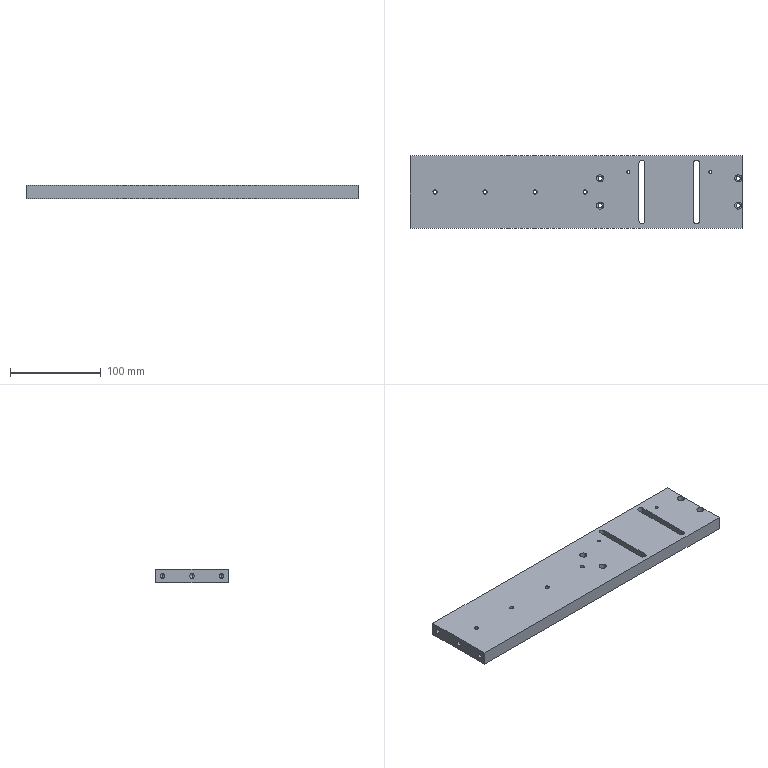Part | SolidWorks | features HoleWzd 6, Extrusion 1 | 1 solid | 88 faces | box 365 x 80 x 15 mm | volume 415130 mm3 | cylinder 54 | plane 24 | cone 10 | commonest cylinder face diameters 4.5 x16 3.3 x8 7.8 x8 8 x8 5 x6 6.6 x4